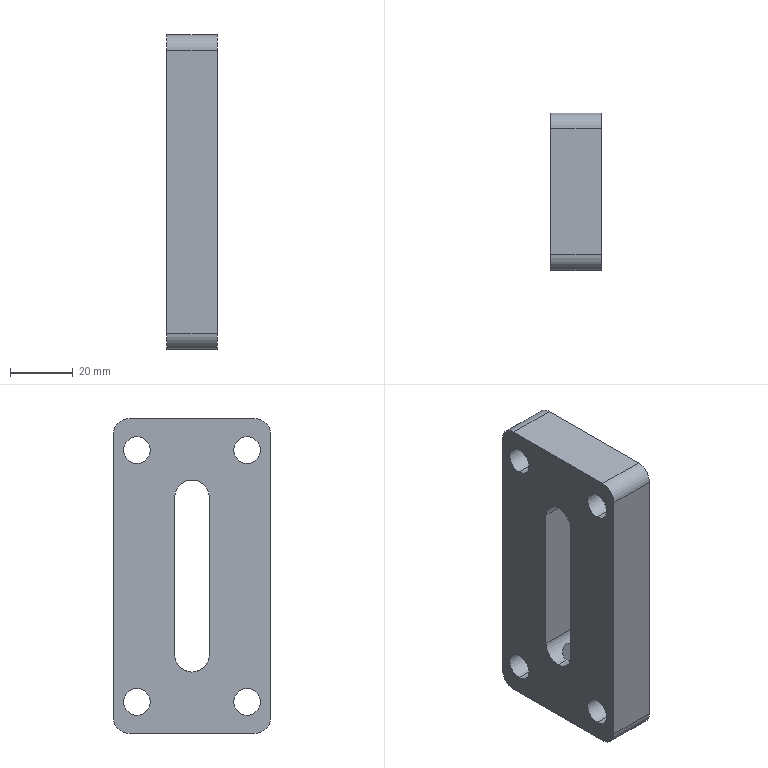Part | SolidWorks | features BaseBody 1 | 1 solid | 25 faces | box 16 x 50 x 100 mm | volume 64572 mm3 | cylinder 17 | plane 8 | commonest cylinder face diameters 8.5 x10 10 x4 11 x3
STEP:
#1=CARTESIAN_POINT('',(-8.,0.,-30.5));
#2=VERTEX_POINT('',#1);
#3=CARTESIAN_POINT('',(-8.,5.5,-25.));
#4=VERTEX_POINT('',#3);
#5=CARTESIAN_POINT('',(-8.,0.,-25.));
#6=DIRECTION('',(1.,0.,0.));
#7=DIRECTION('',(0.,0.,-1.));
#8=AXIS2_PLACEMENT_3D('',#5,#6,#7);
#9=CIRCLE('',#8,5.5);
#10=EDGE_CURVE('',#2,#4,#9,.T.);
#11=ORIENTED_EDGE('',*,*,#10,.F.);
#12=CARTESIAN_POINT('',(-4.25,0.,-30.5));
#13=VERTEX_POINT('',#12);
#14=CARTESIAN_POINT('',(-8.,0.,-30.5));
#15=DIRECTION('',(1.,0.,0.));
#16=VECTOR('',#15,1000.);
#17=LINE('',#14,#16);
#18=EDGE_CURVE('',#2,#13,#17,.T.);
#19=ORIENTED_EDGE('',*,*,#18,.T.);
#20=CARTESIAN_POINT('',(4.25,0.,-30.5));
#21=VERTEX_POINT('',#20);
#22=CARTESIAN_POINT('',(4.25,0.,-30.5));
#23=CARTESIAN_POINT('',(4.25,0.296,-30.5));
#24=CARTESIAN_POINT('',(4.219,0.5849,-30.476));
#25=CARTESIAN_POINT('',(4.102,1.15,-30.386));
#26=CARTESIAN_POINT('',(4.013,1.427,-30.319));
#27=CARTESIAN_POINT('',(3.791,1.941,-30.153));
#28=CARTESIAN_POINT('',(3.656,2.184,-30.054));
#29=CARTESIAN_POINT('',(3.347,2.634,-29.835));
#30=CARTESIAN_POINT('',(3.175,2.838,-29.716));
#31=CARTESIAN_POINT('',(2.796,3.212,-29.47));
#32=CARTESIAN_POINT('',(2.589,3.381,-29.342));
#33=CARTESIAN_POINT('',(2.15,3.675,-29.096));
#34=CARTESIAN_POINT('',(1.917,3.803,-28.976));
#35=CARTESIAN_POINT('',(1.415,4.017,-28.76));
#36=CARTESIAN_POINT('',(1.147,4.102,-28.665));
#37=CARTESIAN_POINT('',(0.5892,4.219,-28.53));
#38=CARTESIAN_POINT('',(0.2935,4.25,-28.491));
#39=CARTESIAN_POINT('',(-0.1431,4.25,-28.491));
#40=CARTESIAN_POINT('',(-0.2886,4.243,-28.5));
#41=CARTESIAN_POINT('',(-0.5795,4.213,-28.536));
#42=CARTESIAN_POINT('',(-0.724,4.19,-28.563));
#43=CARTESIAN_POINT('',(-1.144,4.103,-28.664));
#44=CARTESIAN_POINT('',(-1.413,4.018,-28.759));
#45=CARTESIAN_POINT('',(-1.914,3.804,-28.975));
#46=CARTESIAN_POINT('',(-2.148,3.677,-29.095));
#47=CARTESIAN_POINT('',(-2.588,3.382,-29.342));
#48=CARTESIAN_POINT('',(-2.796,3.212,-29.47));
#49=CARTESIAN_POINT('',(-3.173,2.84,-29.715));
#50=CARTESIAN_POINT('',(-3.345,2.636,-29.834));
#51=CARTESIAN_POINT('',(-3.654,2.187,-30.052));
#52=CARTESIAN_POINT('',(-3.79,1.944,-30.152));
#53=CARTESIAN_POINT('',(-3.956,1.558,-30.276));
#54=CARTESIAN_POINT('',(-4.006,1.426,-30.314));
#55=CARTESIAN_POINT('',(-4.093,1.153,-30.38));
#56=CARTESIAN_POINT('',(-4.13,1.012,-30.408));
#57=CARTESIAN_POINT('',(-4.219,0.5862,-30.476));
#58=CARTESIAN_POINT('',(-4.25,0.2963,-30.5));
#59=CARTESIAN_POINT('',(-4.25,0.,-30.5));
#60=B_SPLINE_CURVE_WITH_KNOTS('',3,(#22,#23,#24,#25,#26,#27,#28,#29,#30,#31,#32,#33,#34,#35,#36,#37,#38,#39,#40,#41,#42,#43,#44,#45,#46,#47,#48,#49,#50,#51,#52,#53,#54,#55,#56,#57,#58,#59),.UNSPECIFIED.,.F.,.F.,(4,2,2,2,2,2,2,2,2,2,2,2,2,2,2,2,2,2,4),(0.,0.0008735,0.001747,0.00262,0.003494,0.004367,0.005241,0.006114,0.006988,0.007424,0.007861,0.008735,0.009608,0.01048,0.01136,0.01223,0.01267,0.0131,0.01398),.UNSPECIFIED.);
#61=EDGE_CURVE('',#21,#13,#60,.T.);
#62=ORIENTED_EDGE('',*,*,#61,.F.);
#63=CARTESIAN_POINT('',(8.,0.,-30.5));
#64=VERTEX_POINT('',#63);
#65=CARTESIAN_POINT('',(-8.,0.,-30.5));
#66=DIRECTION('',(1.,0.,0.));
#67=VECTOR('',#66,1000.);
#68=LINE('',#65,#67);
#69=EDGE_CURVE('',#21,#64,#68,.T.);
#70=ORIENTED_EDGE('',*,*,#69,.T.);
#71=CARTESIAN_POINT('',(8.,5.5,-25.));
#72=VERTEX_POINT('',#71);
#73=CARTESIAN_POINT('',(8.,0.,-25.));
#74=DIRECTION('',(-1.,0.,0.));
#75=DIRECTION('',(0.,0.,-1.));
#76=AXIS2_PLACEMENT_3D('',#73,#74,#75);
#77=CIRCLE('',#76,5.5);
#78=EDGE_CURVE('',#72,#64,#77,.T.);
#79=ORIENTED_EDGE('',*,*,#78,.F.);
#80=CARTESIAN_POINT('',(-8.,5.5,-25.));
#81=DIRECTION('',(-1.,0.,0.));
#82=VECTOR('',#81,1000.);
#83=LINE('',#80,#82);
#84=EDGE_CURVE('',#72,#4,#83,.T.);
#85=ORIENTED_EDGE('',*,*,#84,.T.);
#86=EDGE_LOOP('',(#11,#19,#62,#70,#79,#85));
#87=FACE_OUTER_BOUND('',#86,.T.);
#88=CARTESIAN_POINT('',(-8.,0.,-25.));
#89=DIRECTION('',(1.,0.,0.));
#90=DIRECTION('',(0.,0.,-1.));
#91=AXIS2_PLACEMENT_3D('',#88,#89,#90);
#92=CYLINDRICAL_SURFACE('',#91,5.5);
#93=ADVANCED_FACE('',(#87),#92,.F.);
#94=CARTESIAN_POINT('',(-8.,-17.5,44.25));
#95=VERTEX_POINT('',#94);
#96=CARTESIAN_POINT('',(-8.,-17.5,35.75));
#97=VERTEX_POINT('',#96);
#98=CARTESIAN_POINT('',(-8.,-17.5,40.));
#99=DIRECTION('',(1.,0.,0.));
#100=DIRECTION('',(0.,0.,-1.));
#101=AXIS2_PLACEMENT_3D('',#98,#99,#100);
#102=CIRCLE('',#101,4.25);
#103=EDGE_CURVE('',#95,#97,#102,.T.);
#104=ORIENTED_EDGE('',*,*,#103,.F.);
#105=CARTESIAN_POINT('',(8.,-17.5,44.25));
#106=VERTEX_POINT('',#105);
#107=CARTESIAN_POINT('',(8.,-17.5,44.25));
#108=DIRECTION('',(1.,0.,0.));
#109=VECTOR('',#108,1000.);
#110=LINE('',#107,#109);
#111=EDGE_CURVE('',#95,#106,#110,.T.);
#112=ORIENTED_EDGE('',*,*,#111,.T.);
#113=CARTESIAN_POINT('',(8.,-17.5,35.75));
#114=VERTEX_POINT('',#113);
#115=CARTESIAN_POINT('',(8.,-17.5,40.));
#116=DIRECTION('',(-1.,0.,0.));
#117=DIRECTION('',(0.,0.,-1.));
#118=AXIS2_PLACEMENT_3D('',#115,#116,#117);
#119=CIRCLE('',#118,4.25);
#120=EDGE_CURVE('',#114,#106,#119,.T.);
#121=ORIENTED_EDGE('',*,*,#120,.F.);
#122=CARTESIAN_POINT('',(8.,-17.5,35.75));
#123=DIRECTION('',(1.,0.,0.));
#124=VECTOR('',#123,1000.);
#125=LINE('',#122,#124);
#126=EDGE_CURVE('',#97,#114,#125,.T.);
#127=ORIENTED_EDGE('',*,*,#126,.F.);
#128=EDGE_LOOP('',(#104,#112,#121,#127));
#129=FACE_OUTER_BOUND('',#128,.T.);
#130=CARTESIAN_POINT('',(8.,-17.5,40.));
#131=DIRECTION('',(1.,0.,0.));
#132=DIRECTION('',(0.,0.,-1.));
#133=AXIS2_PLACEMENT_3D('',#130,#131,#132);
#134=CYLINDRICAL_SURFACE('',#133,4.25);
#135=ADVANCED_FACE('',(#129),#134,.F.);
#136=CARTESIAN_POINT('',(-8.,-17.5,-35.75));
#137=VERTEX_POINT('',#136);
#138=CARTESIAN_POINT('',(-8.,-17.5,-44.25));
#139=VERTEX_POINT('',#138);
#140=CARTESIAN_POINT('',(-8.,-17.5,-40.));
#141=DIRECTION('',(1.,0.,0.));
#142=DIRECTION('',(0.,0.,-1.));
#143=AXIS2_PLACEMENT_3D('',#140,#141,#142);
#144=CIRCLE('',#143,4.25);
#145=EDGE_CURVE('',#137,#139,#144,.T.);
#146=ORIENTED_EDGE('',*,*,#145,.F.);
#147=CARTESIAN_POINT('',(8.,-17.5,-35.75));
#148=VERTEX_POINT('',#147);
#149=CARTESIAN_POINT('',(8.,-17.5,-35.75));
#150=DIRECTION('',(1.,0.,0.));
#151=VECTOR('',#150,1000.);
#152=LINE('',#149,#151);
#153=EDGE_CURVE('',#137,#148,#152,.T.);
#154=ORIENTED_EDGE('',*,*,#153,.T.);
#155=CARTESIAN_POINT('',(8.,-17.5,-44.25));
#156=VERTEX_POINT('',#155);
#157=CARTESIAN_POINT('',(8.,-17.5,-40.));
#158=DIRECTION('',(-1.,0.,0.));
#159=DIRECTION('',(0.,0.,-1.));
#160=AXIS2_PLACEMENT_3D('',#157,#158,#159);
#161=CIRCLE('',#160,4.25);
#162=EDGE_CURVE('',#156,#148,#161,.T.);
#163=ORIENTED_EDGE('',*,*,#162,.F.);
#164=CARTESIAN_POINT('',(8.,-17.5,-44.25));
#165=DIRECTION('',(1.,0.,0.));
#166=VECTOR('',#165,1000.);
#167=LINE('',#164,#166);
#168=EDGE_CURVE('',#139,#156,#167,.T.);
#169=ORIENTED_EDGE('',*,*,#168,.F.);
#170=EDGE_LOOP('',(#146,#154,#163,#169));
#171=FACE_OUTER_BOUND('',#170,.T.);
#172=CARTESIAN_POINT('',(8.,-17.5,-40.));
#173=DIRECTION('',(1.,0.,0.));
#174=DIRECTION('',(0.,0.,-1.));
#175=AXIS2_PLACEMENT_3D('',#172,#173,#174);
#176=CYLINDRICAL_SURFACE('',#175,4.25);
#177=ADVANCED_FACE('',(#171),#176,.F.);
#178=CARTESIAN_POINT('',(-8.,17.5,-35.75));
#179=VERTEX_POINT('',#178);
#180=CARTESIAN_POINT('',(-8.,17.5,-44.25));
#181=VERTEX_POINT('',#180);
#182=CARTESIAN_POINT('',(-8.,17.5,-40.));
#183=DIRECTION('',(1.,0.,0.));
#184=DIRECTION('',(0.,0.,-1.));
#185=AXIS2_PLACEMENT_3D('',#182,#183,#184);
#186=CIRCLE('',#185,4.25);
#187=EDGE_CURVE('',#179,#181,#186,.T.);
#188=ORIENTED_EDGE('',*,*,#187,.F.);
#189=CARTESIAN_POINT('',(8.,17.5,-35.75));
#190=VERTEX_POINT('',#189);
#191=CARTESIAN_POINT('',(8.,17.5,-35.75));
#192=DIRECTION('',(1.,0.,0.));
#193=VECTOR('',#192,1000.);
#194=LINE('',#191,#193);
#195=EDGE_CURVE('',#179,#190,#194,.T.);
#196=ORIENTED_EDGE('',*,*,#195,.T.);
#197=CARTESIAN_POINT('',(8.,17.5,-44.25));
#198=VERTEX_POINT('',#197);
#199=CARTESIAN_POINT('',(8.,17.5,-40.));
#200=DIRECTION('',(-1.,0.,0.));
#201=DIRECTION('',(0.,0.,-1.));
#202=AXIS2_PLACEMENT_3D('',#199,#200,#201);
#203=CIRCLE('',#202,4.25);
#204=EDGE_CURVE('',#198,#190,#203,.T.);
#205=ORIENTED_EDGE('',*,*,#204,.F.);
#206=CARTESIAN_POINT('',(8.,17.5,-44.25));
#207=DIRECTION('',(1.,0.,0.));
#208=VECTOR('',#207,1000.);
#209=LINE('',#206,#208);
#210=EDGE_CURVE('',#181,#198,#209,.T.);
#211=ORIENTED_EDGE('',*,*,#210,.F.);
#212=EDGE_LOOP('',(#188,#196,#205,#211));
#213=FACE_OUTER_BOUND('',#212,.T.);
#214=CARTESIAN_POINT('',(8.,17.5,-40.));
#215=DIRECTION('',(1.,0.,0.));
#216=DIRECTION('',(0.,0.,-1.));
#217=AXIS2_PLACEMENT_3D('',#214,#215,#216);
#218=CYLINDRICAL_SURFACE('',#217,4.25);
#219=ADVANCED_FACE('',(#213),#218,.F.);
#220=CARTESIAN_POINT('',(-8.,17.5,44.25));
#221=VERTEX_POINT('',#220);
#222=CARTESIAN_POINT('',(-8.,17.5,35.75));
#223=VERTEX_POINT('',#222);
#224=CARTESIAN_POINT('',(-8.,17.5,40.));
#225=DIRECTION('',(1.,0.,0.));
#226=DIRECTION('',(0.,0.,-1.));
#227=AXIS2_PLACEMENT_3D('',#224,#225,#226);
#228=CIRCLE('',#227,4.25);
#229=EDGE_CURVE('',#221,#223,#228,.T.);
#230=ORIENTED_EDGE('',*,*,#229,.F.);
#231=CARTESIAN_POINT('',(8.,17.5,44.25));
#232=VERTEX_POINT('',#231);
#233=CARTESIAN_POINT('',(8.,17.5,44.25));
#234=DIRECTION('',(1.,0.,0.));
#235=VECTOR('',#234,1000.);
#236=LINE('',#233,#235);
#237=EDGE_CURVE('',#221,#232,#236,.T.);
#238=ORIENTED_EDGE('',*,*,#237,.T.);
#239=CARTESIAN_POINT('',(8.,17.5,35.75));
#240=VERTEX_POINT('',#239);
#241=CARTESIAN_POINT('',(8.,17.5,40.));
#242=DIRECTION('',(-1.,0.,0.));
#243=DIRECTION('',(0.,0.,-1.));
#244=AXIS2_PLACEMENT_3D('',#241,#242,#243);
#245=CIRCLE('',#244,4.25);
#246=EDGE_CURVE('',#240,#232,#245,.T.);
#247=ORIENTED_EDGE('',*,*,#246,.F.);
#248=CARTESIAN_POINT('',(8.,17.5,35.75));
#249=DIRECTION('',(1.,0.,0.));
#250=VECTOR('',#249,1000.);
#251=LINE('',#248,#250);
#252=EDGE_CURVE('',#223,#240,#251,.T.);
#253=ORIENTED_EDGE('',*,*,#252,.F.);
#254=EDGE_LOOP('',(#230,#238,#247,#253));
#255=FACE_OUTER_BOUND('',#254,.T.);
#256=CARTESIAN_POINT('',(8.,17.5,40.));
#257=DIRECTION('',(1.,0.,0.));
#258=DIRECTION('',(0.,0.,-1.));
#259=AXIS2_PLACEMENT_3D('',#256,#257,#258);
#260=CYLINDRICAL_SURFACE('',#259,4.25);
#261=ADVANCED_FACE('',(#255),#260,.F.);
#262=CARTESIAN_POINT('',(-4.25,0.,-30.5));
#263=CARTESIAN_POINT('',(-4.25,-0.296,-30.5));
#264=CARTESIAN_POINT('',(-4.219,-0.5849,-30.476));
#265=CARTESIAN_POINT('',(-4.102,-1.15,-30.386));
#266=CARTESIAN_POINT('',(-4.013,-1.427,-30.319));
#267=CARTESIAN_POINT('',(-3.791,-1.941,-30.153));
#268=CARTESIAN_POINT('',(-3.656,-2.184,-30.054));
#269=CARTESIAN_POINT('',(-3.347,-2.634,-29.835));
#270=CARTESIAN_POINT('',(-3.175,-2.838,-29.716));
#271=CARTESIAN_POINT('',(-2.796,-3.212,-29.47));
#272=CARTESIAN_POINT('',(-2.589,-3.381,-29.342));
#273=CARTESIAN_POINT('',(-2.15,-3.675,-29.096));
#274=CARTESIAN_POINT('',(-1.917,-3.803,-28.976));
#275=CARTESIAN_POINT('',(-1.415,-4.017,-28.76));
#276=CARTESIAN_POINT('',(-1.147,-4.102,-28.665));
#277=CARTESIAN_POINT('',(-0.5892,-4.219,-28.53));
#278=CARTESIAN_POINT('',(-0.2935,-4.25,-28.491));
#279=CARTESIAN_POINT('',(0.1431,-4.25,-28.491));
#280=CARTESIAN_POINT('',(0.2886,-4.243,-28.5));
#281=CARTESIAN_POINT('',(0.5795,-4.213,-28.536));
#282=CARTESIAN_POINT('',(0.724,-4.19,-28.563));
#283=CARTESIAN_POINT('',(1.144,-4.103,-28.664));
#284=CARTESIAN_POINT('',(1.413,-4.018,-28.759));
#285=CARTESIAN_POINT('',(1.914,-3.804,-28.975));
#286=CARTESIAN_POINT('',(2.148,-3.677,-29.095));
#287=CARTESIAN_POINT('',(2.588,-3.382,-29.342));
#288=CARTESIAN_POINT('',(2.796,-3.212,-29.47));
#289=CARTESIAN_POINT('',(3.173,-2.84,-29.715));
#290=CARTESIAN_POINT('',(3.345,-2.636,-29.834));
#291=CARTESIAN_POINT('',(3.654,-2.187,-30.052));
#292=CARTESIAN_POINT('',(3.79,-1.944,-30.152));
#293=CARTESIAN_POINT('',(3.956,-1.558,-30.276));
#294=CARTESIAN_POINT('',(4.006,-1.426,-30.314));
#295=CARTESIAN_POINT('',(4.093,-1.153,-30.38));
#296=CARTESIAN_POINT('',(4.13,-1.012,-30.408));
#297=CARTESIAN_POINT('',(4.219,-0.5862,-30.476));
#298=CARTESIAN_POINT('',(4.25,-0.2957,-30.5));
#299=CARTESIAN_POINT('',(4.25,0.,-30.5));
#300=B_SPLINE_CURVE_WITH_KNOTS('',3,(#262,#263,#264,#265,#266,#267,#268,#269,#270,#271,#272,#273,#274,#275,#276,#277,#278,#279,#280,#281,#282,#283,#284,#285,#286,#287,#288,#289,#290,#291,#292,#293,#294,#295,#296,#297,#298,#299),.UNSPECIFIED.,.F.,.F.,(4,2,2,2,2,2,2,2,2,2,2,2,2,2,2,2,2,2,4),(0.01398,0.01485,0.01572,0.01659,0.01747,0.01834,0.01921,0.02008,0.02096,0.02139,0.02183,0.0227,0.02357,0.02445,0.02532,0.02619,0.02663,0.02706,0.02794),.UNSPECIFIED.);
#301=EDGE_CURVE('',#13,#21,#300,.T.);
#302=ORIENTED_EDGE('',*,*,#301,.T.);
#303=CARTESIAN_POINT('',(4.25,0.,-50.));
#304=VERTEX_POINT('',#303);
#305=CARTESIAN_POINT('',(4.25,0.,-50.));
#306=DIRECTION('',(0.,0.,-1.));
#307=VECTOR('',#306,1000.);
#308=LINE('',#305,#307);
#309=EDGE_CURVE('',#21,#304,#308,.T.);
#310=ORIENTED_EDGE('',*,*,#309,.T.);
#311=CARTESIAN_POINT('',(-4.25,0.,-50.));
#312=VERTEX_POINT('',#311);
#313=CARTESIAN_POINT('',(0.,0.,-50.));
#314=DIRECTION('',(0.,0.,-1.));
#315=DIRECTION('',(-1.,0.,0.));
#316=AXIS2_PLACEMENT_3D('',#313,#314,#315);
#317=CIRCLE('',#316,4.25);
#318=EDGE_CURVE('',#304,#312,#317,.T.);
#319=ORIENTED_EDGE('',*,*,#318,.T.);
#320=CARTESIAN_POINT('',(-4.25,0.,-50.));
#321=DIRECTION('',(0.,0.,-1.));
#322=VECTOR('',#321,1000.);
#323=LINE('',#320,#322);
#324=EDGE_CURVE('',#13,#312,#323,.T.);
#325=ORIENTED_EDGE('',*,*,#324,.F.);
#326=EDGE_LOOP('',(#302,#310,#319,#325));
#327=FACE_OUTER_BOUND('',#326,.T.);
#328=CARTESIAN_POINT('',(0.,0.,-50.));
#329=DIRECTION('',(0.,0.,-1.));
#330=DIRECTION('',(-1.,0.,0.));
#331=AXIS2_PLACEMENT_3D('',#328,#329,#330);
#332=CYLINDRICAL_SURFACE('',#331,4.25);
#333=ADVANCED_FACE('',(#327),#332,.F.);
#334=CARTESIAN_POINT('',(-8.,25.,45.));
#335=VERTEX_POINT('',#334);
#336=CARTESIAN_POINT('',(-8.,25.,-45.));
#337=VERTEX_POINT('',#336);
#338=CARTESIAN_POINT('',(-8.,25.,0.));
#339=DIRECTION('',(0.,0.,-1.));
#340=VECTOR('',#339,1000.);
#341=LINE('',#338,#340);
#342=EDGE_CURVE('',#335,#337,#341,.T.);
#343=ORIENTED_EDGE('',*,*,#342,.T.);
#344=CARTESIAN_POINT('',(-8.,20.,-50.));
#345=VERTEX_POINT('',#344);
#346=CARTESIAN_POINT('',(-8.,20.,-45.));
#347=DIRECTION('',(-1.,0.,0.));
#348=DIRECTION('',(0.,0.,1.));
#349=AXIS2_PLACEMENT_3D('',#346,#347,#348);
#350=CIRCLE('',#349,5.);
#351=EDGE_CURVE('',#337,#345,#350,.T.);
#352=ORIENTED_EDGE('',*,*,#351,.T.);
#353=CARTESIAN_POINT('',(-8.,-20.,-50.));
#354=VERTEX_POINT('',#353);
#355=CARTESIAN_POINT('',(-8.,0.,-50.));
#356=DIRECTION('',(0.,-1.,0.));
#357=VECTOR('',#356,1000.);
#358=LINE('',#355,#357);
#359=EDGE_CURVE('',#345,#354,#358,.T.);
#360=ORIENTED_EDGE('',*,*,#359,.T.);
#361=CARTESIAN_POINT('',(-8.,-25.,-45.));
#362=VERTEX_POINT('',#361);
#363=CARTESIAN_POINT('',(-8.,-20.,-45.));
#364=DIRECTION('',(-1.,0.,0.));
#365=DIRECTION('',(0.,0.,1.));
#366=AXIS2_PLACEMENT_3D('',#363,#364,#365);
#367=CIRCLE('',#366,5.);
#368=EDGE_CURVE('',#354,#362,#367,.T.);
#369=ORIENTED_EDGE('',*,*,#368,.T.);
#370=CARTESIAN_POINT('',(-8.,-25.,45.));
#371=VERTEX_POINT('',#370);
#372=CARTESIAN_POINT('',(-8.,-25.,0.));
#373=DIRECTION('',(0.,0.,1.));
#374=VECTOR('',#373,1000.);
#375=LINE('',#372,#374);
#376=EDGE_CURVE('',#362,#371,#375,.T.);
#377=ORIENTED_EDGE('',*,*,#376,.T.);
#378=CARTESIAN_POINT('',(-8.,-20.,50.));
#379=VERTEX_POINT('',#378);
#380=CARTESIAN_POINT('',(-8.,-20.,45.));
#381=DIRECTION('',(-1.,0.,0.));
#382=DIRECTION('',(0.,0.,1.));
#383=AXIS2_PLACEMENT_3D('',#380,#381,#382);
#384=CIRCLE('',#383,5.);
#385=EDGE_CURVE('',#371,#379,#384,.T.);
#386=ORIENTED_EDGE('',*,*,#385,.T.);
#387=CARTESIAN_POINT('',(-8.,20.,50.));
#388=VERTEX_POINT('',#387);
#389=CARTESIAN_POINT('',(-8.,0.,50.));
#390=DIRECTION('',(0.,1.,0.));
#391=VECTOR('',#390,1000.);
#392=LINE('',#389,#391);
#393=EDGE_CURVE('',#379,#388,#392,.T.);
#394=ORIENTED_EDGE('',*,*,#393,.T.);
#395=CARTESIAN_POINT('',(-8.,20.,45.));
#396=DIRECTION('',(-1.,0.,0.));
#397=DIRECTION('',(0.,0.,1.));
#398=AXIS2_PLACEMENT_3D('',#395,#396,#397);
#399=CIRCLE('',#398,5.);
#400=EDGE_CURVE('',#388,#335,#399,.T.);
#401=ORIENTED_EDGE('',*,*,#400,.T.);
#402=EDGE_LOOP('',(#343,#352,#360,#369,#377,#386,#394,#401));
#403=FACE_OUTER_BOUND('',#402,.T.);
#404=CARTESIAN_POINT('',(-8.,-5.5,-25.));
#405=VERTEX_POINT('',#404);
#406=CARTESIAN_POINT('',(-8.,0.,-25.));
#407=DIRECTION('',(1.,0.,0.));
#408=DIRECTION('',(0.,0.,-1.));
#409=AXIS2_PLACEMENT_3D('',#406,#407,#408);
#410=CIRCLE('',#409,5.5);
#411=EDGE_CURVE('',#405,#2,#410,.T.);
#412=ORIENTED_EDGE('',*,*,#411,.T.);
#413=ORIENTED_EDGE('',*,*,#10,.T.);
#414=CARTESIAN_POINT('',(-8.,5.5,25.));
#415=VERTEX_POINT('',#414);
#416=CARTESIAN_POINT('',(-8.,5.5,0.));
#417=DIRECTION('',(0.,0.,1.));
#418=VECTOR('',#417,1000.);
#419=LINE('',#416,#418);
#420=EDGE_CURVE('',#4,#415,#419,.T.);
#421=ORIENTED_EDGE('',*,*,#420,.T.);
#422=CARTESIAN_POINT('',(-8.,-5.5,25.));
#423=VERTEX_POINT('',#422);
#424=CARTESIAN_POINT('',(-8.,0.,25.));
#425=DIRECTION('',(1.,0.,0.));
#426=DIRECTION('',(0.,0.,-1.));
#427=AXIS2_PLACEMENT_3D('',#424,#425,#426);
#428=CIRCLE('',#427,5.5);
#429=EDGE_CURVE('',#415,#423,#428,.T.);
#430=ORIENTED_EDGE('',*,*,#429,.T.);
#431=CARTESIAN_POINT('',(-8.,-5.5,0.));
#432=DIRECTION('',(0.,0.,-1.));
#433=VECTOR('',#432,1000.);
#434=LINE('',#431,#433);
#435=EDGE_CURVE('',#423,#405,#434,.T.);
#436=ORIENTED_EDGE('',*,*,#435,.T.);
#437=EDGE_LOOP('',(#412,#413,#421,#430,#436));
#438=FACE_BOUND('',#437,.T.);
#439=CARTESIAN_POINT('',(-8.,-17.5,40.));
#440=DIRECTION('',(1.,0.,0.));
#441=DIRECTION('',(0.,0.,-1.));
#442=AXIS2_PLACEMENT_3D('',#439,#440,#441);
#443=CIRCLE('',#442,4.25);
#444=EDGE_CURVE('',#97,#95,#443,.T.);
#445=ORIENTED_EDGE('',*,*,#444,.T.);
#446=ORIENTED_EDGE('',*,*,#103,.T.);
#447=EDGE_LOOP('',(#445,#446));
#448=FACE_BOUND('',#447,.T.);
#449=CARTESIAN_POINT('',(-8.,-17.5,-40.));
#450=DIRECTION('',(1.,0.,0.));
#451=DIRECTION('',(0.,0.,-1.));
#452=AXIS2_PLACEMENT_3D('',#449,#450,#451);
#453=CIRCLE('',#452,4.25);
#454=EDGE_CURVE('',#139,#137,#453,.T.);
#455=ORIENTED_EDGE('',*,*,#454,.T.);
#456=ORIENTED_EDGE('',*,*,#145,.T.);
#457=EDGE_LOOP('',(#455,#456));
#458=FACE_BOUND('',#457,.T.);
#459=CARTESIAN_POINT('',(-8.,17.5,-40.));
#460=DIRECTION('',(1.,0.,0.));
#461=DIRECTION('',(0.,0.,-1.));
#462=AXIS2_PLACEMENT_3D('',#459,#460,#461);
#463=CIRCLE('',#462,4.25);
#464=EDGE_CURVE('',#181,#179,#463,.T.);
#465=ORIENTED_EDGE('',*,*,#464,.T.);
#466=ORIENTED_EDGE('',*,*,#187,.T.);
#467=EDGE_LOOP('',(#465,#466));
#468=FACE_BOUND('',#467,.T.);
#469=CARTESIAN_POINT('',(-8.,17.5,40.));
#470=DIRECTION('',(1.,0.,0.));
#471=DIRECTION('',(0.,0.,-1.));
#472=AXIS2_PLACEMENT_3D('',#469,#470,#471);
#473=CIRCLE('',#472,4.25);
#474=EDGE_CURVE('',#223,#221,#473,.T.);
#475=ORIENTED_EDGE('',*,*,#474,.T.);
#476=ORIENTED_EDGE('',*,*,#229,.T.);
#477=EDGE_LOOP('',(#475,#476));
#478=FACE_BOUND('',#477,.T.);
#479=CARTESIAN_POINT('',(-8.,0.,0.));
#480=DIRECTION('',(-1.,0.,0.));
#481=DIRECTION('',(0.,0.,1.));
#482=AXIS2_PLACEMENT_3D('',#479,#480,#481);
#483=PLANE('',#482);
#484=ADVANCED_FACE('',(#403,#438,#448,#458,#468,#478),#483,.T.);
#485=ORIENTED_EDGE('',*,*,#351,.F.);
#486=CARTESIAN_POINT('',(8.,25.,-45.));
#487=VERTEX_POINT('',#486);
#488=CARTESIAN_POINT('',(8.,25.,-45.));
#489=DIRECTION('',(1.,0.,0.));
#490=VECTOR('',#489,1000.);
#491=LINE('',#488,#490);
#492=EDGE_CURVE('',#337,#487,#491,.T.);
#493=ORIENTED_EDGE('',*,*,#492,.T.);
#494=CARTESIAN_POINT('',(8.,20.,-50.));
#495=VERTEX_POINT('',#494);
#496=CARTESIAN_POINT('',(8.,20.,-45.));
#497=DIRECTION('',(-1.,0.,0.));
#498=DIRECTION('',(0.,0.,1.));
#499=AXIS2_PLACEMENT_3D('',#496,#497,#498);
#500=CIRCLE('',#499,5.);
#501=EDGE_CURVE('',#487,#495,#500,.T.);
#502=ORIENTED_EDGE('',*,*,#501,.T.);
#503=CARTESIAN_POINT('',(8.,20.,-50.));
#504=DIRECTION('',(-1.,0.,0.));
#505=VECTOR('',#504,1000.);
#506=LINE('',#503,#505);
#507=EDGE_CURVE('',#495,#345,#506,.T.);
#508=ORIENTED_EDGE('',*,*,#507,.T.);
#509=EDGE_LOOP('',(#485,#493,#502,#508));
#510=FACE_OUTER_BOUND('',#509,.T.);
#511=CARTESIAN_POINT('',(8.,20.,-45.));
#512=DIRECTION('',(-1.,0.,0.));
#513=DIRECTION('',(0.,0.,1.));
#514=AXIS2_PLACEMENT_3D('',#511,#512,#513);
#515=CYLINDRICAL_SURFACE('',#514,5.);
#516=ADVANCED_FACE('',(#510),#515,.T.);
#517=ORIENTED_EDGE('',*,*,#492,.F.);
#518=ORIENTED_EDGE('',*,*,#342,.F.);
#519=CARTESIAN_POINT('',(8.,25.,45.));
#520=VERTEX_POINT('',#519);
#521=CARTESIAN_POINT('',(8.,25.,45.));
#522=DIRECTION('',(-1.,0.,0.));
#523=VECTOR('',#522,1000.);
#524=LINE('',#521,#523);
#525=EDGE_CURVE('',#520,#335,#524,.T.);
#526=ORIENTED_EDGE('',*,*,#525,.F.);
#527=CARTESIAN_POINT('',(8.,25.,50.));
#528=DIRECTION('',(0.,0.,1.));
#529=VECTOR('',#528,1000.);
#530=LINE('',#527,#529);
#531=EDGE_CURVE('',#487,#520,#530,.T.);
#532=ORIENTED_EDGE('',*,*,#531,.F.);
#533=EDGE_LOOP('',(#517,#518,#526,#532));
#534=FACE_OUTER_BOUND('',#533,.T.);
#535=CARTESIAN_POINT('',(8.,25.,50.));
#536=DIRECTION('',(0.,-1.,0.));
#537=DIRECTION('',(0.,0.,-1.));
#538=AXIS2_PLACEMENT_3D('',#535,#536,#537);
#539=PLANE('',#538);
#540=ADVANCED_FACE('',(#534),#539,.F.);
#541=ORIENTED_EDGE('',*,*,#400,.F.);
#542=CARTESIAN_POINT('',(8.,20.,50.));
#543=VERTEX_POINT('',#542);
#544=CARTESIAN_POINT('',(8.,20.,50.));
#545=DIRECTION('',(1.,0.,0.));
#546=VECTOR('',#545,1000.);
#547=LINE('',#544,#546);
#548=EDGE_CURVE('',#388,#543,#547,.T.);
#549=ORIENTED_EDGE('',*,*,#548,.T.);
#550=CARTESIAN_POINT('',(8.,20.,45.));
#551=DIRECTION('',(-1.,0.,0.));
#552=DIRECTION('',(0.,0.,1.));
#553=AXIS2_PLACEMENT_3D('',#550,#551,#552);
#554=CIRCLE('',#553,5.);
#555=EDGE_CURVE('',#543,#520,#554,.T.);
#556=ORIENTED_EDGE('',*,*,#555,.T.);
#557=ORIENTED_EDGE('',*,*,#525,.T.);
#558=EDGE_LOOP('',(#541,#549,#556,#557));
#559=FACE_OUTER_BOUND('',#558,.T.);
#560=CARTESIAN_POINT('',(8.,20.,45.));
#561=DIRECTION('',(-1.,0.,0.));
#562=DIRECTION('',(0.,0.,1.));
#563=AXIS2_PLACEMENT_3D('',#560,#561,#562);
#564=CYLINDRICAL_SURFACE('',#563,5.);
#565=ADVANCED_FACE('',(#559),#564,.T.);
#566=CARTESIAN_POINT('',(8.,-20.,50.));
#567=VERTEX_POINT('',#566);
#568=CARTESIAN_POINT('',(8.,-20.,50.));
#569=DIRECTION('',(-1.,0.,0.));
#570=VECTOR('',#569,1000.);
#571=LINE('',#568,#570);
#572=EDGE_CURVE('',#567,#379,#571,.T.);
#573=ORIENTED_EDGE('',*,*,#572,.F.);
#574=CARTESIAN_POINT('',(8.,-25.,50.));
#575=DIRECTION('',(0.,-1.,0.));
#576=VECTOR('',#575,1000.);
#577=LINE('',#574,#576);
#578=EDGE_CURVE('',#543,#567,#577,.T.);
#579=ORIENTED_EDGE('',*,*,#578,.F.);
#580=ORIENTED_EDGE('',*,*,#548,.F.);
#581=ORIENTED_EDGE('',*,*,#393,.F.);
#582=EDGE_LOOP('',(#573,#579,#580,#581));
#583=FACE_OUTER_BOUND('',#582,.T.);
#584=CARTESIAN_POINT('',(8.,-25.,50.));
#585=DIRECTION('',(0.,0.,-1.));
#586=DIRECTION('',(-1.,0.,0.));
#587=AXIS2_PLACEMENT_3D('',#584,#585,#586);
#588=PLANE('',#587);
#589=ADVANCED_FACE('',(#583),#588,.F.);
#590=ORIENTED_EDGE('',*,*,#385,.F.);
#591=CARTESIAN_POINT('',(8.,-25.,45.));
#592=VERTEX_POINT('',#591);
#593=CARTESIAN_POINT('',(8.,-25.,45.));
#594=DIRECTION('',(1.,0.,0.));
#595=VECTOR('',#594,1000.);
#596=LINE('',#593,#595);
#597=EDGE_CURVE('',#371,#592,#596,.T.);
#598=ORIENTED_EDGE('',*,*,#597,.T.);
#599=CARTESIAN_POINT('',(8.,-20.,45.));
#600=DIRECTION('',(-1.,0.,0.));
#601=DIRECTION('',(0.,0.,1.));
#602=AXIS2_PLACEMENT_3D('',#599,#600,#601);
#603=CIRCLE('',#602,5.);
#604=EDGE_CURVE('',#592,#567,#603,.T.);
#605=ORIENTED_EDGE('',*,*,#604,.T.);
#606=ORIENTED_EDGE('',*,*,#572,.T.);
#607=EDGE_LOOP('',(#590,#598,#605,#606));
#608=FACE_OUTER_BOUND('',#607,.T.);
#609=CARTESIAN_POINT('',(8.,-20.,45.));
#610=DIRECTION('',(-1.,0.,0.));
#611=DIRECTION('',(0.,0.,1.));
#612=AXIS2_PLACEMENT_3D('',#609,#610,#611);
#613=CYLINDRICAL_SURFACE('',#612,5.);
#614=ADVANCED_FACE('',(#608),#613,.T.);
#615=CARTESIAN_POINT('',(8.,-25.,-45.));
#616=VERTEX_POINT('',#615);
#617=CARTESIAN_POINT('',(8.,-25.,-45.));
#618=DIRECTION('',(-1.,0.,0.));
#619=VECTOR('',#618,1000.);
#620=LINE('',#617,#619);
#621=EDGE_CURVE('',#616,#362,#620,.T.);
#622=ORIENTED_EDGE('',*,*,#621,.F.);
#623=CARTESIAN_POINT('',(8.,-25.,50.));
#624=DIRECTION('',(0.,0.,-1.));
#625=VECTOR('',#624,1000.);
#626=LINE('',#623,#625);
#627=EDGE_CURVE('',#592,#616,#626,.T.);
#628=ORIENTED_EDGE('',*,*,#627,.F.);
#629=ORIENTED_EDGE('',*,*,#597,.F.);
#630=ORIENTED_EDGE('',*,*,#376,.F.);
#631=EDGE_LOOP('',(#622,#628,#629,#630));
#632=FACE_OUTER_BOUND('',#631,.T.);
#633=CARTESIAN_POINT('',(8.,-25.,50.));
#634=DIRECTION('',(0.,1.,0.));
#635=DIRECTION('',(0.,0.,1.));
#636=AXIS2_PLACEMENT_3D('',#633,#634,#635);
#637=PLANE('',#636);
#638=ADVANCED_FACE('',(#632),#637,.F.);
#639=ORIENTED_EDGE('',*,*,#368,.F.);
#640=CARTESIAN_POINT('',(8.,-20.,-50.));
#641=VERTEX_POINT('',#640);
#642=CARTESIAN_POINT('',(8.,-20.,-50.));
#643=DIRECTION('',(1.,0.,0.));
#644=VECTOR('',#643,1000.);
#645=LINE('',#642,#644);
#646=EDGE_CURVE('',#354,#641,#645,.T.);
#647=ORIENTED_EDGE('',*,*,#646,.T.);
#648=CARTESIAN_POINT('',(8.,-20.,-45.));
#649=DIRECTION('',(-1.,0.,0.));
#650=DIRECTION('',(0.,0.,1.));
#651=AXIS2_PLACEMENT_3D('',#648,#649,#650);
#652=CIRCLE('',#651,5.);
#653=EDGE_CURVE('',#641,#616,#652,.T.);
#654=ORIENTED_EDGE('',*,*,#653,.T.);
#655=ORIENTED_EDGE('',*,*,#621,.T.);
#656=EDGE_LOOP('',(#639,#647,#654,#655));
#657=FACE_OUTER_BOUND('',#656,.T.);
#658=CARTESIAN_POINT('',(8.,-20.,-45.));
#659=DIRECTION('',(-1.,0.,0.));
#660=DIRECTION('',(0.,0.,1.));
#661=AXIS2_PLACEMENT_3D('',#658,#659,#660);
#662=CYLINDRICAL_SURFACE('',#661,5.);
#663=ADVANCED_FACE('',(#657),#662,.T.);
#664=ORIENTED_EDGE('',*,*,#646,.F.);
#665=ORIENTED_EDGE('',*,*,#359,.F.);
#666=ORIENTED_EDGE('',*,*,#507,.F.);
#667=CARTESIAN_POINT('',(8.,-25.,-50.));
#668=DIRECTION('',(0.,1.,0.));
#669=VECTOR('',#668,1000.);
#670=LINE('',#667,#669);
#671=EDGE_CURVE('',#641,#495,#670,.T.);
#672=ORIENTED_EDGE('',*,*,#671,.F.);
#673=EDGE_LOOP('',(#664,#665,#666,#672));
#674=FACE_OUTER_BOUND('',#673,.T.);
#675=CARTESIAN_POINT('',(0.,0.,-50.));
#676=DIRECTION('',(0.,0.,-1.));
#677=DIRECTION('',(-1.,0.,0.));
#678=AXIS2_PLACEMENT_3D('',#675,#676,#677);
#679=CIRCLE('',#678,4.25);
#680=EDGE_CURVE('',#312,#304,#679,.T.);
#681=ORIENTED_EDGE('',*,*,#680,.F.);
#682=ORIENTED_EDGE('',*,*,#318,.F.);
#683=EDGE_LOOP('',(#681,#682));
#684=FACE_BOUND('',#683,.T.);
#685=CARTESIAN_POINT('',(8.,-25.,-50.));
#686=DIRECTION('',(0.,0.,1.));
#687=DIRECTION('',(1.,0.,0.));
#688=AXIS2_PLACEMENT_3D('',#685,#686,#687);
#689=PLANE('',#688);
#690=ADVANCED_FACE('',(#674,#684),#689,.F.);
#691=CARTESIAN_POINT('',(8.,5.5,25.));
#692=VERTEX_POINT('',#691);
#693=CARTESIAN_POINT('',(-8.,5.5,25.));
#694=DIRECTION('',(1.,0.,0.));
#695=VECTOR('',#694,1000.);
#696=LINE('',#693,#695);
#697=EDGE_CURVE('',#415,#692,#696,.T.);
#698=ORIENTED_EDGE('',*,*,#697,.F.);
#699=ORIENTED_EDGE('',*,*,#420,.F.);
#700=ORIENTED_EDGE('',*,*,#84,.F.);
#701=CARTESIAN_POINT('',(8.,5.5,25.));
#702=DIRECTION('',(0.,0.,-1.));
#703=VECTOR('',#702,1000.);
#704=LINE('',#701,#703);
#705=EDGE_CURVE('',#692,#72,#704,.T.);
#706=ORIENTED_EDGE('',*,*,#705,.F.);
#707=EDGE_LOOP('',(#698,#699,#700,#706));
#708=FACE_OUTER_BOUND('',#707,.T.);
#709=CARTESIAN_POINT('',(-8.,5.5,25.));
#710=DIRECTION('',(0.,1.,0.));
#711=DIRECTION('',(0.,0.,1.));
#712=AXIS2_PLACEMENT_3D('',#709,#710,#711);
#713=PLANE('',#712);
#714=ADVANCED_FACE('',(#708),#713,.F.);
#715=ORIENTED_EDGE('',*,*,#18,.F.);
#716=ORIENTED_EDGE('',*,*,#411,.F.);
#717=CARTESIAN_POINT('',(8.,-5.5,-25.));
#718=VERTEX_POINT('',#717);
#719=CARTESIAN_POINT('',(-8.,-5.5,-25.));
#720=DIRECTION('',(-1.,0.,0.));
#721=VECTOR('',#720,1000.);
#722=LINE('',#719,#721);
#723=EDGE_CURVE('',#718,#405,#722,.T.);
#724=ORIENTED_EDGE('',*,*,#723,.F.);
#725=CARTESIAN_POINT('',(8.,0.,-25.));
#726=DIRECTION('',(-1.,0.,0.));
#727=DIRECTION('',(0.,0.,-1.));
#728=AXIS2_PLACEMENT_3D('',#725,#726,#727);
#729=CIRCLE('',#728,5.5);
#730=EDGE_CURVE('',#64,#718,#729,.T.);
#731=ORIENTED_EDGE('',*,*,#730,.F.);
#732=ORIENTED_EDGE('',*,*,#69,.F.);
#733=ORIENTED_EDGE('',*,*,#301,.F.);
#734=EDGE_LOOP('',(#715,#716,#724,#731,#732,#733));
#735=FACE_OUTER_BOUND('',#734,.T.);
#736=CARTESIAN_POINT('',(-8.,0.,-25.));
#737=DIRECTION('',(1.,0.,0.));
#738=DIRECTION('',(0.,0.,-1.));
#739=AXIS2_PLACEMENT_3D('',#736,#737,#738);
#740=CYLINDRICAL_SURFACE('',#739,5.5);
#741=ADVANCED_FACE('',(#735),#740,.F.);
#742=ORIENTED_EDGE('',*,*,#723,.T.);
#743=ORIENTED_EDGE('',*,*,#435,.F.);
#744=CARTESIAN_POINT('',(8.,-5.5,25.));
#745=VERTEX_POINT('',#744);
#746=CARTESIAN_POINT('',(-8.,-5.5,25.));
#747=DIRECTION('',(-1.,0.,0.));
#748=VECTOR('',#747,1000.);
#749=LINE('',#746,#748);
#750=EDGE_CURVE('',#745,#423,#749,.T.);
#751=ORIENTED_EDGE('',*,*,#750,.F.);
#752=CARTESIAN_POINT('',(8.,-5.5,25.));
#753=DIRECTION('',(0.,0.,1.));
#754=VECTOR('',#753,1000.);
#755=LINE('',#752,#754);
#756=EDGE_CURVE('',#718,#745,#755,.T.);
#757=ORIENTED_EDGE('',*,*,#756,.F.);
#758=EDGE_LOOP('',(#742,#743,#751,#757));
#759=FACE_OUTER_BOUND('',#758,.T.);
#760=CARTESIAN_POINT('',(-8.,-5.5,25.));
#761=DIRECTION('',(0.,-1.,0.));
#762=DIRECTION('',(0.,0.,-1.));
#763=AXIS2_PLACEMENT_3D('',#760,#761,#762);
#764=PLANE('',#763);
#765=ADVANCED_FACE('',(#759),#764,.F.);
#766=ORIENTED_EDGE('',*,*,#750,.T.);
#767=ORIENTED_EDGE('',*,*,#429,.F.);
#768=ORIENTED_EDGE('',*,*,#697,.T.);
#769=CARTESIAN_POINT('',(8.,0.,25.));
#770=DIRECTION('',(-1.,0.,0.));
#771=DIRECTION('',(0.,0.,-1.));
#772=AXIS2_PLACEMENT_3D('',#769,#770,#771);
#773=CIRCLE('',#772,5.5);
#774=EDGE_CURVE('',#745,#692,#773,.T.);
#775=ORIENTED_EDGE('',*,*,#774,.F.);
#776=EDGE_LOOP('',(#766,#767,#768,#775));
#777=FACE_OUTER_BOUND('',#776,.T.);
#778=CARTESIAN_POINT('',(-8.,0.,25.));
#779=DIRECTION('',(1.,0.,0.));
#780=DIRECTION('',(0.,0.,-1.));
#781=AXIS2_PLACEMENT_3D('',#778,#779,#780);
#782=CYLINDRICAL_SURFACE('',#781,5.5);
#783=ADVANCED_FACE('',(#777),#782,.F.);
#784=ORIENTED_EDGE('',*,*,#111,.F.);
#785=ORIENTED_EDGE('',*,*,#444,.F.);
#786=ORIENTED_EDGE('',*,*,#126,.T.);
#787=CARTESIAN_POINT('',(8.,-17.5,40.));
#788=DIRECTION('',(-1.,0.,0.));
#789=DIRECTION('',(0.,0.,-1.));
#790=AXIS2_PLACEMENT_3D('',#787,#788,#789);
#791=CIRCLE('',#790,4.25);
#792=EDGE_CURVE('',#106,#114,#791,.T.);
#793=ORIENTED_EDGE('',*,*,#792,.F.);
#794=EDGE_LOOP('',(#784,#785,#786,#793));
#795=FACE_OUTER_BOUND('',#794,.T.);
#796=CARTESIAN_POINT('',(8.,-17.5,40.));
#797=DIRECTION('',(1.,0.,0.));
#798=DIRECTION('',(0.,0.,-1.));
#799=AXIS2_PLACEMENT_3D('',#796,#797,#798);
#800=CYLINDRICAL_SURFACE('',#799,4.25);
#801=ADVANCED_FACE('',(#795),#800,.F.);
#802=ORIENTED_EDGE('',*,*,#153,.F.);
#803=ORIENTED_EDGE('',*,*,#454,.F.);
#804=ORIENTED_EDGE('',*,*,#168,.T.);
#805=CARTESIAN_POINT('',(8.,-17.5,-40.));
#806=DIRECTION('',(-1.,0.,0.));
#807=DIRECTION('',(0.,0.,-1.));
#808=AXIS2_PLACEMENT_3D('',#805,#806,#807);
#809=CIRCLE('',#808,4.25);
#810=EDGE_CURVE('',#148,#156,#809,.T.);
#811=ORIENTED_EDGE('',*,*,#810,.F.);
#812=EDGE_LOOP('',(#802,#803,#804,#811));
#813=FACE_OUTER_BOUND('',#812,.T.);
#814=CARTESIAN_POINT('',(8.,-17.5,-40.));
#815=DIRECTION('',(1.,0.,0.));
#816=DIRECTION('',(0.,0.,-1.));
#817=AXIS2_PLACEMENT_3D('',#814,#815,#816);
#818=CYLINDRICAL_SURFACE('',#817,4.25);
#819=ADVANCED_FACE('',(#813),#818,.F.);
#820=ORIENTED_EDGE('',*,*,#195,.F.);
#821=ORIENTED_EDGE('',*,*,#464,.F.);
#822=ORIENTED_EDGE('',*,*,#210,.T.);
#823=CARTESIAN_POINT('',(8.,17.5,-40.));
#824=DIRECTION('',(-1.,0.,0.));
#825=DIRECTION('',(0.,0.,-1.));
#826=AXIS2_PLACEMENT_3D('',#823,#824,#825);
#827=CIRCLE('',#826,4.25);
#828=EDGE_CURVE('',#190,#198,#827,.T.);
#829=ORIENTED_EDGE('',*,*,#828,.F.);
#830=EDGE_LOOP('',(#820,#821,#822,#829));
#831=FACE_OUTER_BOUND('',#830,.T.);
#832=CARTESIAN_POINT('',(8.,17.5,-40.));
#833=DIRECTION('',(1.,0.,0.));
#834=DIRECTION('',(0.,0.,-1.));
#835=AXIS2_PLACEMENT_3D('',#832,#833,#834);
#836=CYLINDRICAL_SURFACE('',#835,4.25);
#837=ADVANCED_FACE('',(#831),#836,.F.);
#838=ORIENTED_EDGE('',*,*,#237,.F.);
#839=ORIENTED_EDGE('',*,*,#474,.F.);
#840=ORIENTED_EDGE('',*,*,#252,.T.);
#841=CARTESIAN_POINT('',(8.,17.5,40.));
#842=DIRECTION('',(-1.,0.,0.));
#843=DIRECTION('',(0.,0.,-1.));
#844=AXIS2_PLACEMENT_3D('',#841,#842,#843);
#845=CIRCLE('',#844,4.25);
#846=EDGE_CURVE('',#232,#240,#845,.T.);
#847=ORIENTED_EDGE('',*,*,#846,.F.);
#848=EDGE_LOOP('',(#838,#839,#840,#847));
#849=FACE_OUTER_BOUND('',#848,.T.);
#850=CARTESIAN_POINT('',(8.,17.5,40.));
#851=DIRECTION('',(1.,0.,0.));
#852=DIRECTION('',(0.,0.,-1.));
#853=AXIS2_PLACEMENT_3D('',#850,#851,#852);
#854=CYLINDRICAL_SURFACE('',#853,4.25);
#855=ADVANCED_FACE('',(#849),#854,.F.);
#856=ORIENTED_EDGE('',*,*,#653,.F.);
#857=ORIENTED_EDGE('',*,*,#671,.T.);
#858=ORIENTED_EDGE('',*,*,#501,.F.);
#859=ORIENTED_EDGE('',*,*,#531,.T.);
#860=ORIENTED_EDGE('',*,*,#555,.F.);
#861=ORIENTED_EDGE('',*,*,#578,.T.);
#862=ORIENTED_EDGE('',*,*,#604,.F.);
#863=ORIENTED_EDGE('',*,*,#627,.T.);
#864=EDGE_LOOP('',(#856,#857,#858,#859,#860,#861,#862,#863));
#865=FACE_OUTER_BOUND('',#864,.T.);
#866=ORIENTED_EDGE('',*,*,#774,.T.);
#867=ORIENTED_EDGE('',*,*,#705,.T.);
#868=ORIENTED_EDGE('',*,*,#78,.T.);
#869=ORIENTED_EDGE('',*,*,#730,.T.);
#870=ORIENTED_EDGE('',*,*,#756,.T.);
#871=EDGE_LOOP('',(#866,#867,#868,#869,#870));
#872=FACE_BOUND('',#871,.T.);
#873=ORIENTED_EDGE('',*,*,#120,.T.);
#874=ORIENTED_EDGE('',*,*,#792,.T.);
#875=EDGE_LOOP('',(#873,#874));
#876=FACE_BOUND('',#875,.T.);
#877=ORIENTED_EDGE('',*,*,#162,.T.);
#878=ORIENTED_EDGE('',*,*,#810,.T.);
#879=EDGE_LOOP('',(#877,#878));
#880=FACE_BOUND('',#879,.T.);
#881=ORIENTED_EDGE('',*,*,#204,.T.);
#882=ORIENTED_EDGE('',*,*,#828,.T.);
#883=EDGE_LOOP('',(#881,#882));
#884=FACE_BOUND('',#883,.T.);
#885=ORIENTED_EDGE('',*,*,#246,.T.);
#886=ORIENTED_EDGE('',*,*,#846,.T.);
#887=EDGE_LOOP('',(#885,#886));
#888=FACE_BOUND('',#887,.T.);
#889=CARTESIAN_POINT('',(8.,0.,0.));
#890=DIRECTION('',(-1.,0.,0.));
#891=DIRECTION('',(0.,0.,1.));
#892=AXIS2_PLACEMENT_3D('',#889,#890,#891);
#893=PLANE('',#892);
#894=ADVANCED_FACE('',(#865,#872,#876,#880,#884,#888),#893,.F.);
#895=ORIENTED_EDGE('',*,*,#309,.F.);
#896=ORIENTED_EDGE('',*,*,#61,.T.);
#897=ORIENTED_EDGE('',*,*,#324,.T.);
#898=ORIENTED_EDGE('',*,*,#680,.T.);
#899=EDGE_LOOP('',(#895,#896,#897,#898));
#900=FACE_OUTER_BOUND('',#899,.T.);
#901=CARTESIAN_POINT('',(0.,0.,-50.));
#902=DIRECTION('',(0.,0.,-1.));
#903=DIRECTION('',(-1.,0.,0.));
#904=AXIS2_PLACEMENT_3D('',#901,#902,#903);
#905=CYLINDRICAL_SURFACE('',#904,4.25);
#906=ADVANCED_FACE('',(#900),#905,.F.);
#907=CLOSED_SHELL('',(#93,#135,#177,#219,#261,#333,#484,#516,#540,#565,#589,#614,#638,#663,#690,#714,#741,#765,#783,#801,#819,#837,#855,#894,#906));
#908=MANIFOLD_SOLID_BREP('',#907);
#909=CARTESIAN_POINT('',(0.,0.,0.));
#910=DIRECTION('',(0.,0.,1.));
#911=DIRECTION('',(1.,0.,0.));
#912=AXIS2_PLACEMENT_3D('',#909,#910,#911);
#913=(LENGTH_UNIT()NAMED_UNIT(*)SI_UNIT(.MILLI.,.METRE.));
#914=UNCERTAINTY_MEASURE_WITH_UNIT(LENGTH_MEASURE(0.00001),#913,'','');
#915=(NAMED_UNIT(*)PLANE_ANGLE_UNIT()SI_UNIT($,.RADIAN.));
#916=(NAMED_UNIT(*)SI_UNIT($,.STERADIAN.)SOLID_ANGLE_UNIT());
#917=(GEOMETRIC_REPRESENTATION_CONTEXT(3)GLOBAL_UNCERTAINTY_ASSIGNED_CONTEXT((#914))GLOBAL_UNIT_ASSIGNED_CONTEXT((#913,#915,#916))REPRESENTATION_CONTEXT('',''));
#918=ADVANCED_BREP_SHAPE_REPRESENTATION('',(#908,#912),#917);